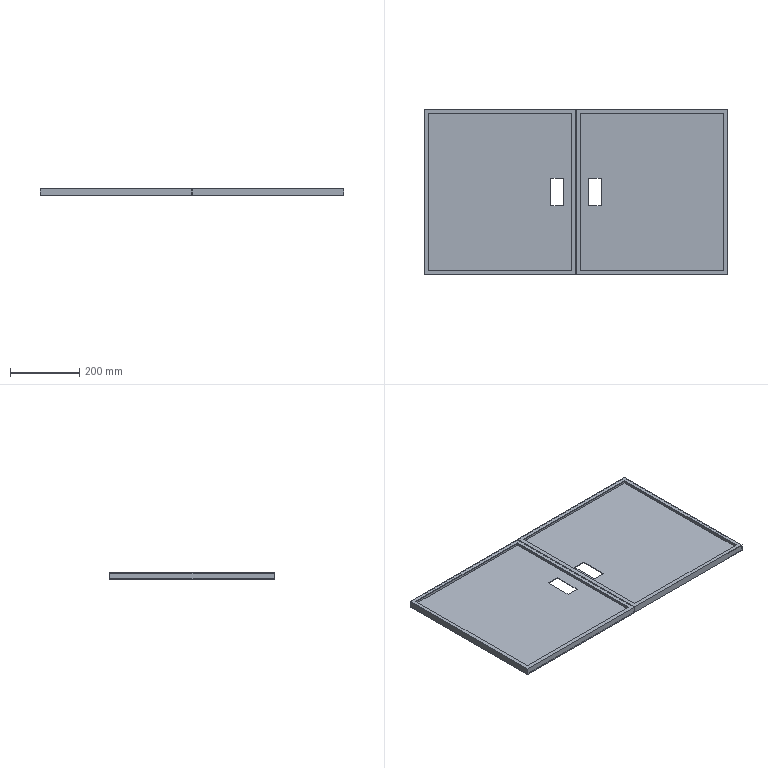Part | STEP file | Door | 2 solids | 40 faces | box 880 x 480 x 20 mm | volume 1033932 mm3 | plane 40